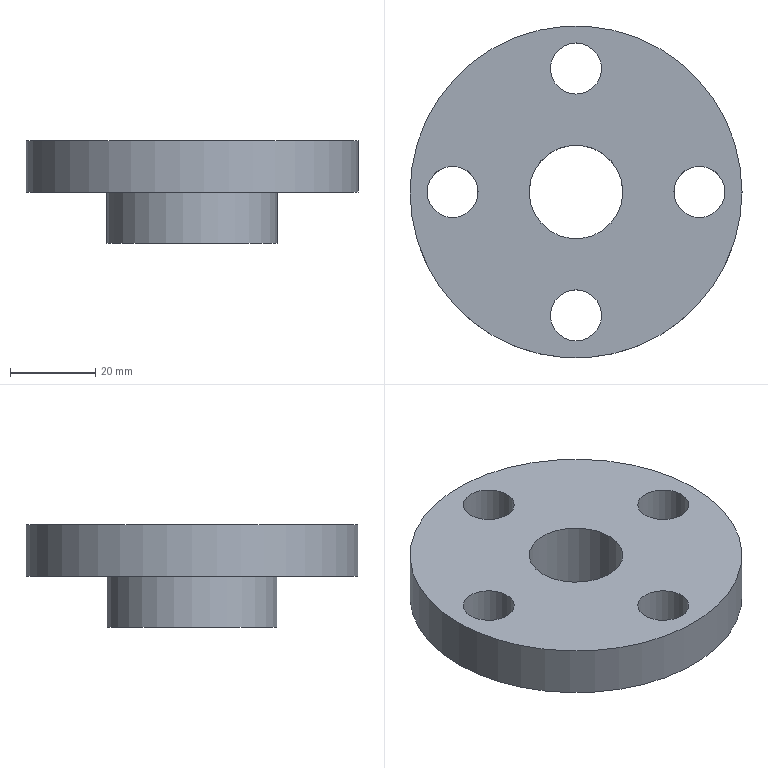CAM job | NX | 3-axis milling, drilling | part box 78 x 78 x 24 mm | stock box 78 x 78 x 24 mm
Tools:
number,name,description,diameter,corner_radius,flute_length,length,flutes
1,ZXZ,Milling Tool-5 Parameters,6.0,0.0,50.0,75.0,2
7,D6A45,Milling Tool-5 Parameters,6.0,0.0,3.0,3.0,2
2,12.0ZT,Drilling Tool,12.0,0.0,35.0,50.0,2
Operations:
program,operation,operation_type,tool,method,geometry_group,spindle_rpm,surface_speed,feed_per_tooth,feed_cut,feed_plunge,cut_length_mm,path_length_mm,cut_time_min,machine_time_min
1,DRILLING,Operation,ZXZ,METHOD,A,3000.0,56.0,0.0333,200.0,0.0,16.0,224.365,0.08,0.1008
1,DRILLING_COPY,Operation,12.0ZT,METHOD,A,800.0,30.0,0.0938,150.0,0.0,80.421,353.207,0.5361,0.5634
1,ZLEVEL_PROFILE_1_COPY_1,ZLevelMilling,D6A45,METHOD,A,7500.0,141.0,0.0667,1000.0,100.0,151.68,549.841,0.1517,0.1915